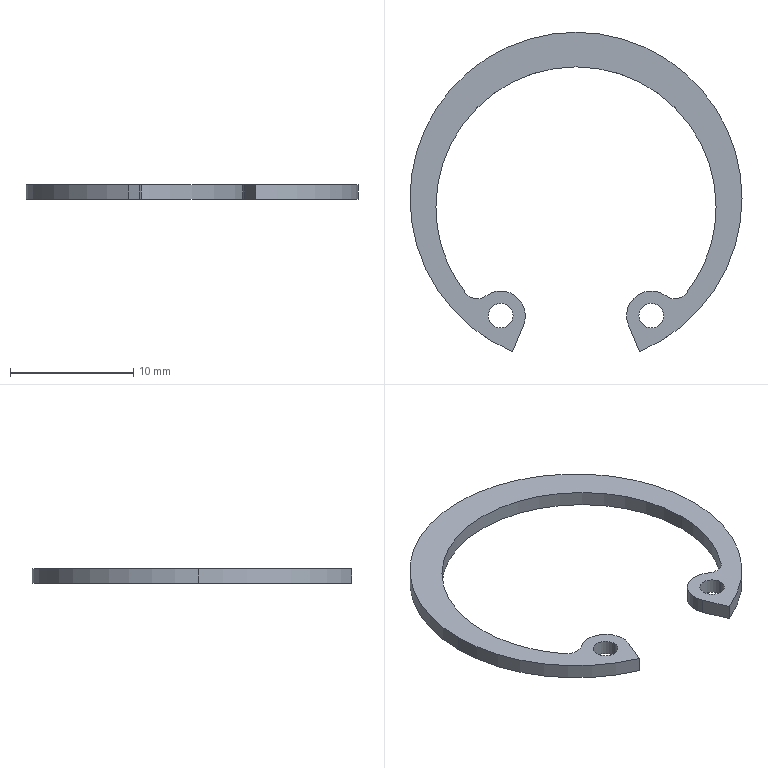Part | STEP file | circlips for holes--type a gb(GB_CONNECTING_PIECE_RING_RRH 25) | 1 solid | 19 faces | box 26.9 x 25.876 x 1.2 mm | volume 193.354 mm3 | cylinder 15 | plane 4 | commonest cylinder face diameters 2 x4 4 x3 22.7 x3 26.9 x3 2.4 x2
STEP:
#1=CARTESIAN_POINT('',(-7.104,-9.51,-1.2));
#2=VERTEX_POINT('',#1);
#3=CARTESIAN_POINT('',(-5.104,-9.51,-1.2));
#4=VERTEX_POINT('',#3);
#5=CARTESIAN_POINT('',(-6.104,-9.51,-1.2));
#6=DIRECTION('',(0.,0.,1.));
#7=DIRECTION('',(1.,0.,0.));
#8=AXIS2_PLACEMENT_3D('',#5,#6,#7);
#9=CIRCLE('',#8,1.);
#10=EDGE_CURVE('',#2,#4,#9,.T.);
#11=ORIENTED_EDGE('',*,*,#10,.F.);
#12=CARTESIAN_POINT('',(-7.104,-9.51,0.));
#13=VERTEX_POINT('',#12);
#14=CARTESIAN_POINT('',(-7.104,-9.51,-1.2));
#15=DIRECTION('',(0.,0.,1.));
#16=VECTOR('',#15,1000.);
#17=LINE('',#14,#16);
#18=EDGE_CURVE('',#2,#13,#17,.T.);
#19=ORIENTED_EDGE('',*,*,#18,.T.);
#20=CARTESIAN_POINT('',(-5.104,-9.51,0.));
#21=VERTEX_POINT('',#20);
#22=CARTESIAN_POINT('',(-6.104,-9.51,0.));
#23=DIRECTION('',(0.,0.,1.));
#24=DIRECTION('',(1.,0.,0.));
#25=AXIS2_PLACEMENT_3D('',#22,#23,#24);
#26=CIRCLE('',#25,1.);
#27=EDGE_CURVE('',#13,#21,#26,.T.);
#28=ORIENTED_EDGE('',*,*,#27,.T.);
#29=CARTESIAN_POINT('',(-5.104,-9.51,-1.2));
#30=DIRECTION('',(0.,0.,1.));
#31=VECTOR('',#30,1000.);
#32=LINE('',#29,#31);
#33=EDGE_CURVE('',#4,#21,#32,.T.);
#34=ORIENTED_EDGE('',*,*,#33,.F.);
#35=EDGE_LOOP('',(#11,#19,#28,#34));
#36=FACE_OUTER_BOUND('',#35,.T.);
#37=CARTESIAN_POINT('',(-6.104,-9.51,-1.2));
#38=DIRECTION('',(0.,0.,1.));
#39=DIRECTION('',(1.,0.,0.));
#40=AXIS2_PLACEMENT_3D('',#37,#38,#39);
#41=CYLINDRICAL_SURFACE('',#40,1.);
#42=ADVANCED_FACE('',(#36),#41,.F.);
#43=CARTESIAN_POINT('',(5.104,-9.51,-1.2));
#44=VERTEX_POINT('',#43);
#45=CARTESIAN_POINT('',(7.104,-9.51,-1.2));
#46=VERTEX_POINT('',#45);
#47=CARTESIAN_POINT('',(6.104,-9.51,-1.2));
#48=DIRECTION('',(0.,0.,1.));
#49=DIRECTION('',(-1.,0.,0.));
#50=AXIS2_PLACEMENT_3D('',#47,#48,#49);
#51=CIRCLE('',#50,1.);
#52=EDGE_CURVE('',#44,#46,#51,.T.);
#53=ORIENTED_EDGE('',*,*,#52,.F.);
#54=CARTESIAN_POINT('',(5.104,-9.51,0.));
#55=VERTEX_POINT('',#54);
#56=CARTESIAN_POINT('',(5.104,-9.51,-1.2));
#57=DIRECTION('',(0.,0.,1.));
#58=VECTOR('',#57,1000.);
#59=LINE('',#56,#58);
#60=EDGE_CURVE('',#44,#55,#59,.T.);
#61=ORIENTED_EDGE('',*,*,#60,.T.);
#62=CARTESIAN_POINT('',(7.104,-9.51,0.));
#63=VERTEX_POINT('',#62);
#64=CARTESIAN_POINT('',(6.104,-9.51,0.));
#65=DIRECTION('',(0.,0.,1.));
#66=DIRECTION('',(-1.,0.,0.));
#67=AXIS2_PLACEMENT_3D('',#64,#65,#66);
#68=CIRCLE('',#67,1.);
#69=EDGE_CURVE('',#55,#63,#68,.T.);
#70=ORIENTED_EDGE('',*,*,#69,.T.);
#71=CARTESIAN_POINT('',(7.104,-9.51,-1.2));
#72=DIRECTION('',(0.,0.,1.));
#73=VECTOR('',#72,1000.);
#74=LINE('',#71,#73);
#75=EDGE_CURVE('',#46,#63,#74,.T.);
#76=ORIENTED_EDGE('',*,*,#75,.F.);
#77=EDGE_LOOP('',(#53,#61,#70,#76));
#78=FACE_OUTER_BOUND('',#77,.T.);
#79=CARTESIAN_POINT('',(6.104,-9.51,-1.2));
#80=DIRECTION('',(0.,0.,1.));
#81=DIRECTION('',(1.,0.,0.));
#82=AXIS2_PLACEMENT_3D('',#79,#80,#81);
#83=CYLINDRICAL_SURFACE('',#82,1.);
#84=ADVANCED_FACE('',(#78),#83,.F.);
#85=CARTESIAN_POINT('',(-4.256,-10.275,-1.2));
#86=VERTEX_POINT('',#85);
#87=CARTESIAN_POINT('',(-4.104,-9.51,-1.2));
#88=VERTEX_POINT('',#87);
#89=CARTESIAN_POINT('',(-6.104,-9.51,-1.2));
#90=DIRECTION('',(0.,0.,1.));
#91=DIRECTION('',(1.,0.,0.));
#92=AXIS2_PLACEMENT_3D('',#89,#90,#91);
#93=CIRCLE('',#92,2.);
#94=EDGE_CURVE('',#86,#88,#93,.T.);
#95=ORIENTED_EDGE('',*,*,#94,.T.);
#96=CARTESIAN_POINT('',(-4.104,-9.51,0.));
#97=VERTEX_POINT('',#96);
#98=CARTESIAN_POINT('',(-4.104,-9.51,-1.2));
#99=DIRECTION('',(0.,0.,1.));
#100=VECTOR('',#99,1000.);
#101=LINE('',#98,#100);
#102=EDGE_CURVE('',#88,#97,#101,.T.);
#103=ORIENTED_EDGE('',*,*,#102,.T.);
#104=CARTESIAN_POINT('',(-4.256,-10.275,0.));
#105=VERTEX_POINT('',#104);
#106=CARTESIAN_POINT('',(-6.104,-9.51,0.));
#107=DIRECTION('',(0.,0.,1.));
#108=DIRECTION('',(1.,0.,0.));
#109=AXIS2_PLACEMENT_3D('',#106,#107,#108);
#110=CIRCLE('',#109,2.);
#111=EDGE_CURVE('',#105,#97,#110,.T.);
#112=ORIENTED_EDGE('',*,*,#111,.F.);
#113=CARTESIAN_POINT('',(-4.256,-10.275,-1.2));
#114=DIRECTION('',(0.,0.,1.));
#115=VECTOR('',#114,1000.);
#116=LINE('',#113,#115);
#117=EDGE_CURVE('',#86,#105,#116,.T.);
#118=ORIENTED_EDGE('',*,*,#117,.F.);
#119=EDGE_LOOP('',(#95,#103,#112,#118));
#120=FACE_OUTER_BOUND('',#119,.T.);
#121=CARTESIAN_POINT('',(-6.104,-9.51,-1.2));
#122=DIRECTION('',(0.,0.,1.));
#123=DIRECTION('',(1.,0.,0.));
#124=AXIS2_PLACEMENT_3D('',#121,#122,#123);
#125=CYLINDRICAL_SURFACE('',#124,2.);
#126=ADVANCED_FACE('',(#120),#125,.T.);
#127=CARTESIAN_POINT('',(-8.954,-7.675,-1.2));
#128=VERTEX_POINT('',#127);
#129=CARTESIAN_POINT('',(-11.35,-0.7,-1.2));
#130=VERTEX_POINT('',#129);
#131=CARTESIAN_POINT('',(0.,-0.7,-1.2));
#132=DIRECTION('',(0.,0.,-1.));
#133=DIRECTION('',(1.,0.,0.));
#134=AXIS2_PLACEMENT_3D('',#131,#132,#133);
#135=CIRCLE('',#134,11.35);
#136=EDGE_CURVE('',#128,#130,#135,.T.);
#137=ORIENTED_EDGE('',*,*,#136,.T.);
#138=CARTESIAN_POINT('',(-11.35,-0.7,0.));
#139=VERTEX_POINT('',#138);
#140=CARTESIAN_POINT('',(-11.35,-0.7,-1.2));
#141=DIRECTION('',(0.,0.,1.));
#142=VECTOR('',#141,1000.);
#143=LINE('',#140,#142);
#144=EDGE_CURVE('',#130,#139,#143,.T.);
#145=ORIENTED_EDGE('',*,*,#144,.T.);
#146=CARTESIAN_POINT('',(-8.954,-7.675,0.));
#147=VERTEX_POINT('',#146);
#148=CARTESIAN_POINT('',(0.,-0.7,0.));
#149=DIRECTION('',(0.,0.,-1.));
#150=DIRECTION('',(1.,0.,0.));
#151=AXIS2_PLACEMENT_3D('',#148,#149,#150);
#152=CIRCLE('',#151,11.35);
#153=EDGE_CURVE('',#147,#139,#152,.T.);
#154=ORIENTED_EDGE('',*,*,#153,.F.);
#155=CARTESIAN_POINT('',(-8.954,-7.675,-1.2));
#156=DIRECTION('',(0.,0.,1.));
#157=VECTOR('',#156,1000.);
#158=LINE('',#155,#157);
#159=EDGE_CURVE('',#128,#147,#158,.T.);
#160=ORIENTED_EDGE('',*,*,#159,.F.);
#161=EDGE_LOOP('',(#137,#145,#154,#160));
#162=FACE_OUTER_BOUND('',#161,.T.);
#163=CARTESIAN_POINT('',(0.,-0.7,-1.2));
#164=DIRECTION('',(0.,0.,1.));
#165=DIRECTION('',(1.,0.,0.));
#166=AXIS2_PLACEMENT_3D('',#163,#164,#165);
#167=CYLINDRICAL_SURFACE('',#166,11.35);
#168=ADVANCED_FACE('',(#162),#167,.F.);
#169=ORIENTED_EDGE('',*,*,#144,.F.);
#170=CARTESIAN_POINT('',(11.35,-0.7,-1.2));
#171=VERTEX_POINT('',#170);
#172=CARTESIAN_POINT('',(0.,-0.7,-1.2));
#173=DIRECTION('',(0.,0.,-1.));
#174=DIRECTION('',(1.,0.,0.));
#175=AXIS2_PLACEMENT_3D('',#172,#173,#174);
#176=CIRCLE('',#175,11.35);
#177=EDGE_CURVE('',#130,#171,#176,.T.);
#178=ORIENTED_EDGE('',*,*,#177,.T.);
#179=CARTESIAN_POINT('',(11.35,-0.7,0.));
#180=VERTEX_POINT('',#179);
#181=CARTESIAN_POINT('',(11.35,-0.7,-1.2));
#182=DIRECTION('',(0.,0.,1.));
#183=VECTOR('',#182,1000.);
#184=LINE('',#181,#183);
#185=EDGE_CURVE('',#171,#180,#184,.T.);
#186=ORIENTED_EDGE('',*,*,#185,.T.);
#187=CARTESIAN_POINT('',(0.,-0.7,0.));
#188=DIRECTION('',(0.,0.,-1.));
#189=DIRECTION('',(1.,0.,0.));
#190=AXIS2_PLACEMENT_3D('',#187,#188,#189);
#191=CIRCLE('',#190,11.35);
#192=EDGE_CURVE('',#139,#180,#191,.T.);
#193=ORIENTED_EDGE('',*,*,#192,.F.);
#194=EDGE_LOOP('',(#169,#178,#186,#193));
#195=FACE_OUTER_BOUND('',#194,.T.);
#196=CARTESIAN_POINT('',(0.,-0.7,-1.2));
#197=DIRECTION('',(0.,0.,1.));
#198=DIRECTION('',(1.,0.,0.));
#199=AXIS2_PLACEMENT_3D('',#196,#197,#198);
#200=CYLINDRICAL_SURFACE('',#199,11.35);
#201=ADVANCED_FACE('',(#195),#200,.F.);
#202=CARTESIAN_POINT('',(13.45,0.,-1.2));
#203=VERTEX_POINT('',#202);
#204=CARTESIAN_POINT('',(-13.45,0.,-1.2));
#205=VERTEX_POINT('',#204);
#206=CARTESIAN_POINT('',(0.,0.,-1.2));
#207=DIRECTION('',(0.,0.,1.));
#208=DIRECTION('',(1.,0.,0.));
#209=AXIS2_PLACEMENT_3D('',#206,#207,#208);
#210=CIRCLE('',#209,13.45);
#211=EDGE_CURVE('',#203,#205,#210,.T.);
#212=ORIENTED_EDGE('',*,*,#211,.T.);
#213=CARTESIAN_POINT('',(-13.45,0.,0.));
#214=VERTEX_POINT('',#213);
#215=CARTESIAN_POINT('',(-13.45,0.,-1.2));
#216=DIRECTION('',(0.,0.,1.));
#217=VECTOR('',#216,1000.);
#218=LINE('',#215,#217);
#219=EDGE_CURVE('',#205,#214,#218,.T.);
#220=ORIENTED_EDGE('',*,*,#219,.T.);
#221=CARTESIAN_POINT('',(13.45,0.,0.));
#222=VERTEX_POINT('',#221);
#223=CARTESIAN_POINT('',(0.,0.,0.));
#224=DIRECTION('',(0.,0.,1.));
#225=DIRECTION('',(1.,0.,0.));
#226=AXIS2_PLACEMENT_3D('',#223,#224,#225);
#227=CIRCLE('',#226,13.45);
#228=EDGE_CURVE('',#222,#214,#227,.T.);
#229=ORIENTED_EDGE('',*,*,#228,.F.);
#230=CARTESIAN_POINT('',(13.45,0.,-1.2));
#231=DIRECTION('',(0.,0.,1.));
#232=VECTOR('',#231,1000.);
#233=LINE('',#230,#232);
#234=EDGE_CURVE('',#203,#222,#233,.T.);
#235=ORIENTED_EDGE('',*,*,#234,.F.);
#236=EDGE_LOOP('',(#212,#220,#229,#235));
#237=FACE_OUTER_BOUND('',#236,.T.);
#238=CARTESIAN_POINT('',(0.,0.,-1.2));
#239=DIRECTION('',(0.,0.,1.));
#240=DIRECTION('',(1.,0.,0.));
#241=AXIS2_PLACEMENT_3D('',#238,#239,#240);
#242=CYLINDRICAL_SURFACE('',#241,13.45);
#243=ADVANCED_FACE('',(#237),#242,.T.);
#244=CARTESIAN_POINT('',(5.147,-12.426,-1.2));
#245=VERTEX_POINT('',#244);
#246=CARTESIAN_POINT('',(0.,0.,-1.2));
#247=DIRECTION('',(0.,0.,1.));
#248=DIRECTION('',(1.,0.,0.));
#249=AXIS2_PLACEMENT_3D('',#246,#247,#248);
#250=CIRCLE('',#249,13.45);
#251=EDGE_CURVE('',#245,#203,#250,.T.);
#252=ORIENTED_EDGE('',*,*,#251,.T.);
#253=ORIENTED_EDGE('',*,*,#234,.T.);
#254=CARTESIAN_POINT('',(5.147,-12.426,0.));
#255=VERTEX_POINT('',#254);
#256=CARTESIAN_POINT('',(0.,0.,0.));
#257=DIRECTION('',(0.,0.,1.));
#258=DIRECTION('',(1.,0.,0.));
#259=AXIS2_PLACEMENT_3D('',#256,#257,#258);
#260=CIRCLE('',#259,13.45);
#261=EDGE_CURVE('',#255,#222,#260,.T.);
#262=ORIENTED_EDGE('',*,*,#261,.F.);
#263=CARTESIAN_POINT('',(5.147,-12.426,-1.2));
#264=DIRECTION('',(0.,0.,1.));
#265=VECTOR('',#264,1000.);
#266=LINE('',#263,#265);
#267=EDGE_CURVE('',#245,#255,#266,.T.);
#268=ORIENTED_EDGE('',*,*,#267,.F.);
#269=EDGE_LOOP('',(#252,#253,#262,#268));
#270=FACE_OUTER_BOUND('',#269,.T.);
#271=CARTESIAN_POINT('',(0.,0.,-1.2));
#272=DIRECTION('',(0.,0.,1.));
#273=DIRECTION('',(1.,0.,0.));
#274=AXIS2_PLACEMENT_3D('',#271,#272,#273);
#275=CYLINDRICAL_SURFACE('',#274,13.45);
#276=ADVANCED_FACE('',(#270),#275,.T.);
#277=ORIENTED_EDGE('',*,*,#219,.F.);
#278=CARTESIAN_POINT('',(-5.147,-12.426,-1.2));
#279=VERTEX_POINT('',#278);
#280=CARTESIAN_POINT('',(0.,0.,-1.2));
#281=DIRECTION('',(0.,0.,1.));
#282=DIRECTION('',(1.,0.,0.));
#283=AXIS2_PLACEMENT_3D('',#280,#281,#282);
#284=CIRCLE('',#283,13.45);
#285=EDGE_CURVE('',#205,#279,#284,.T.);
#286=ORIENTED_EDGE('',*,*,#285,.T.);
#287=CARTESIAN_POINT('',(-5.147,-12.426,0.));
#288=VERTEX_POINT('',#287);
#289=CARTESIAN_POINT('',(-5.147,-12.426,-1.2));
#290=DIRECTION('',(0.,0.,1.));
#291=VECTOR('',#290,1000.);
#292=LINE('',#289,#291);
#293=EDGE_CURVE('',#279,#288,#292,.T.);
#294=ORIENTED_EDGE('',*,*,#293,.T.);
#295=CARTESIAN_POINT('',(0.,0.,0.));
#296=DIRECTION('',(0.,0.,1.));
#297=DIRECTION('',(1.,0.,0.));
#298=AXIS2_PLACEMENT_3D('',#295,#296,#297);
#299=CIRCLE('',#298,13.45);
#300=EDGE_CURVE('',#214,#288,#299,.T.);
#301=ORIENTED_EDGE('',*,*,#300,.F.);
#302=EDGE_LOOP('',(#277,#286,#294,#301));
#303=FACE_OUTER_BOUND('',#302,.T.);
#304=CARTESIAN_POINT('',(0.,0.,-1.2));
#305=DIRECTION('',(0.,0.,1.));
#306=DIRECTION('',(1.,0.,0.));
#307=AXIS2_PLACEMENT_3D('',#304,#305,#306);
#308=CYLINDRICAL_SURFACE('',#307,13.45);
#309=ADVANCED_FACE('',(#303),#308,.T.);
#310=CARTESIAN_POINT('',(4.256,-10.275,0.));
#311=VERTEX_POINT('',#310);
#312=CARTESIAN_POINT('',(4.256,-10.275,0.));
#313=DIRECTION('',(0.3827,-0.9239,0.));
#314=VECTOR('',#313,1000.);
#315=LINE('',#312,#314);
#316=EDGE_CURVE('',#311,#255,#315,.T.);
#317=ORIENTED_EDGE('',*,*,#316,.F.);
#318=CARTESIAN_POINT('',(4.256,-10.275,-1.2));
#319=VERTEX_POINT('',#318);
#320=CARTESIAN_POINT('',(4.256,-10.275,-1.2));
#321=DIRECTION('',(0.,0.,1.));
#322=VECTOR('',#321,1000.);
#323=LINE('',#320,#322);
#324=EDGE_CURVE('',#319,#311,#323,.T.);
#325=ORIENTED_EDGE('',*,*,#324,.F.);
#326=CARTESIAN_POINT('',(4.256,-10.275,-1.2));
#327=DIRECTION('',(0.3827,-0.9239,0.));
#328=VECTOR('',#327,1000.);
#329=LINE('',#326,#328);
#330=EDGE_CURVE('',#319,#245,#329,.T.);
#331=ORIENTED_EDGE('',*,*,#330,.T.);
#332=ORIENTED_EDGE('',*,*,#267,.T.);
#333=EDGE_LOOP('',(#317,#325,#331,#332));
#334=FACE_OUTER_BOUND('',#333,.T.);
#335=CARTESIAN_POINT('',(4.256,-10.275,-1.2));
#336=DIRECTION('',(-0.9239,-0.3827,0.));
#337=DIRECTION('',(0.3827,-0.9239,0.));
#338=AXIS2_PLACEMENT_3D('',#335,#336,#337);
#339=PLANE('',#338);
#340=ADVANCED_FACE('',(#334),#339,.T.);
#341=CARTESIAN_POINT('',(7.294,-7.902,0.));
#342=VERTEX_POINT('',#341);
#343=CARTESIAN_POINT('',(6.104,-9.51,0.));
#344=DIRECTION('',(0.,0.,1.));
#345=DIRECTION('',(-1.,0.,0.));
#346=AXIS2_PLACEMENT_3D('',#343,#344,#345);
#347=CIRCLE('',#346,2.);
#348=EDGE_CURVE('',#342,#311,#347,.T.);
#349=ORIENTED_EDGE('',*,*,#348,.F.);
#350=CARTESIAN_POINT('',(7.294,-7.902,-1.2));
#351=VERTEX_POINT('',#350);
#352=CARTESIAN_POINT('',(7.294,-7.902,-1.2));
#353=DIRECTION('',(0.,0.,1.));
#354=VECTOR('',#353,1000.);
#355=LINE('',#352,#354);
#356=EDGE_CURVE('',#351,#342,#355,.T.);
#357=ORIENTED_EDGE('',*,*,#356,.F.);
#358=CARTESIAN_POINT('',(6.104,-9.51,-1.2));
#359=DIRECTION('',(0.,0.,1.));
#360=DIRECTION('',(-1.,0.,0.));
#361=AXIS2_PLACEMENT_3D('',#358,#359,#360);
#362=CIRCLE('',#361,2.);
#363=EDGE_CURVE('',#351,#319,#362,.T.);
#364=ORIENTED_EDGE('',*,*,#363,.T.);
#365=ORIENTED_EDGE('',*,*,#324,.T.);
#366=EDGE_LOOP('',(#349,#357,#364,#365));
#367=FACE_OUTER_BOUND('',#366,.T.);
#368=CARTESIAN_POINT('',(6.104,-9.51,-1.2));
#369=DIRECTION('',(0.,0.,1.));
#370=DIRECTION('',(1.,0.,0.));
#371=AXIS2_PLACEMENT_3D('',#368,#369,#370);
#372=CYLINDRICAL_SURFACE('',#371,2.);
#373=ADVANCED_FACE('',(#367),#372,.T.);
#374=CARTESIAN_POINT('',(8.954,-7.675,0.));
#375=VERTEX_POINT('',#374);
#376=CARTESIAN_POINT('',(8.007,-6.937,0.));
#377=DIRECTION('',(0.,0.,-1.));
#378=DIRECTION('',(-1.,0.,0.));
#379=AXIS2_PLACEMENT_3D('',#376,#377,#378);
#380=CIRCLE('',#379,1.2);
#381=EDGE_CURVE('',#375,#342,#380,.T.);
#382=ORIENTED_EDGE('',*,*,#381,.F.);
#383=CARTESIAN_POINT('',(8.954,-7.675,-1.2));
#384=VERTEX_POINT('',#383);
#385=CARTESIAN_POINT('',(8.954,-7.675,-1.2));
#386=DIRECTION('',(0.,0.,1.));
#387=VECTOR('',#386,1000.);
#388=LINE('',#385,#387);
#389=EDGE_CURVE('',#384,#375,#388,.T.);
#390=ORIENTED_EDGE('',*,*,#389,.F.);
#391=CARTESIAN_POINT('',(8.007,-6.937,-1.2));
#392=DIRECTION('',(0.,0.,-1.));
#393=DIRECTION('',(-1.,0.,0.));
#394=AXIS2_PLACEMENT_3D('',#391,#392,#393);
#395=CIRCLE('',#394,1.2);
#396=EDGE_CURVE('',#384,#351,#395,.T.);
#397=ORIENTED_EDGE('',*,*,#396,.T.);
#398=ORIENTED_EDGE('',*,*,#356,.T.);
#399=EDGE_LOOP('',(#382,#390,#397,#398));
#400=FACE_OUTER_BOUND('',#399,.T.);
#401=CARTESIAN_POINT('',(8.007,-6.937,-1.2));
#402=DIRECTION('',(0.,0.,1.));
#403=DIRECTION('',(1.,0.,0.));
#404=AXIS2_PLACEMENT_3D('',#401,#402,#403);
#405=CYLINDRICAL_SURFACE('',#404,1.2);
#406=ADVANCED_FACE('',(#400),#405,.F.);
#407=ORIENTED_EDGE('',*,*,#185,.F.);
#408=CARTESIAN_POINT('',(0.,-0.7,-1.2));
#409=DIRECTION('',(0.,0.,-1.));
#410=DIRECTION('',(1.,0.,0.));
#411=AXIS2_PLACEMENT_3D('',#408,#409,#410);
#412=CIRCLE('',#411,11.35);
#413=EDGE_CURVE('',#171,#384,#412,.T.);
#414=ORIENTED_EDGE('',*,*,#413,.T.);
#415=ORIENTED_EDGE('',*,*,#389,.T.);
#416=CARTESIAN_POINT('',(0.,-0.7,0.));
#417=DIRECTION('',(0.,0.,-1.));
#418=DIRECTION('',(1.,0.,0.));
#419=AXIS2_PLACEMENT_3D('',#416,#417,#418);
#420=CIRCLE('',#419,11.35);
#421=EDGE_CURVE('',#180,#375,#420,.T.);
#422=ORIENTED_EDGE('',*,*,#421,.F.);
#423=EDGE_LOOP('',(#407,#414,#415,#422));
#424=FACE_OUTER_BOUND('',#423,.T.);
#425=CARTESIAN_POINT('',(0.,-0.7,-1.2));
#426=DIRECTION('',(0.,0.,1.));
#427=DIRECTION('',(1.,0.,0.));
#428=AXIS2_PLACEMENT_3D('',#425,#426,#427);
#429=CYLINDRICAL_SURFACE('',#428,11.35);
#430=ADVANCED_FACE('',(#424),#429,.F.);
#431=CARTESIAN_POINT('',(-7.294,-7.902,0.));
#432=VERTEX_POINT('',#431);
#433=CARTESIAN_POINT('',(-8.007,-6.937,0.));
#434=DIRECTION('',(0.,0.,-1.));
#435=DIRECTION('',(1.,0.,0.));
#436=AXIS2_PLACEMENT_3D('',#433,#434,#435);
#437=CIRCLE('',#436,1.2);
#438=EDGE_CURVE('',#432,#147,#437,.T.);
#439=ORIENTED_EDGE('',*,*,#438,.F.);
#440=CARTESIAN_POINT('',(-7.294,-7.902,-1.2));
#441=VERTEX_POINT('',#440);
#442=CARTESIAN_POINT('',(-7.294,-7.902,-1.2));
#443=DIRECTION('',(0.,0.,1.));
#444=VECTOR('',#443,1000.);
#445=LINE('',#442,#444);
#446=EDGE_CURVE('',#441,#432,#445,.T.);
#447=ORIENTED_EDGE('',*,*,#446,.F.);
#448=CARTESIAN_POINT('',(-8.007,-6.937,-1.2));
#449=DIRECTION('',(0.,0.,-1.));
#450=DIRECTION('',(1.,0.,0.));
#451=AXIS2_PLACEMENT_3D('',#448,#449,#450);
#452=CIRCLE('',#451,1.2);
#453=EDGE_CURVE('',#441,#128,#452,.T.);
#454=ORIENTED_EDGE('',*,*,#453,.T.);
#455=ORIENTED_EDGE('',*,*,#159,.T.);
#456=EDGE_LOOP('',(#439,#447,#454,#455));
#457=FACE_OUTER_BOUND('',#456,.T.);
#458=CARTESIAN_POINT('',(-8.007,-6.937,-1.2));
#459=DIRECTION('',(0.,0.,1.));
#460=DIRECTION('',(1.,0.,0.));
#461=AXIS2_PLACEMENT_3D('',#458,#459,#460);
#462=CYLINDRICAL_SURFACE('',#461,1.2);
#463=ADVANCED_FACE('',(#457),#462,.F.);
#464=ORIENTED_EDGE('',*,*,#102,.F.);
#465=CARTESIAN_POINT('',(-6.104,-9.51,-1.2));
#466=DIRECTION('',(0.,0.,1.));
#467=DIRECTION('',(1.,0.,0.));
#468=AXIS2_PLACEMENT_3D('',#465,#466,#467);
#469=CIRCLE('',#468,2.);
#470=EDGE_CURVE('',#88,#441,#469,.T.);
#471=ORIENTED_EDGE('',*,*,#470,.T.);
#472=ORIENTED_EDGE('',*,*,#446,.T.);
#473=CARTESIAN_POINT('',(-6.104,-9.51,0.));
#474=DIRECTION('',(0.,0.,1.));
#475=DIRECTION('',(1.,0.,0.));
#476=AXIS2_PLACEMENT_3D('',#473,#474,#475);
#477=CIRCLE('',#476,2.);
#478=EDGE_CURVE('',#97,#432,#477,.T.);
#479=ORIENTED_EDGE('',*,*,#478,.F.);
#480=EDGE_LOOP('',(#464,#471,#472,#479));
#481=FACE_OUTER_BOUND('',#480,.T.);
#482=CARTESIAN_POINT('',(-6.104,-9.51,-1.2));
#483=DIRECTION('',(0.,0.,1.));
#484=DIRECTION('',(1.,0.,0.));
#485=AXIS2_PLACEMENT_3D('',#482,#483,#484);
#486=CYLINDRICAL_SURFACE('',#485,2.);
#487=ADVANCED_FACE('',(#481),#486,.T.);
#488=CARTESIAN_POINT('',(-4.256,-10.275,0.));
#489=DIRECTION('',(0.3827,0.9239,0.));
#490=VECTOR('',#489,1000.);
#491=LINE('',#488,#490);
#492=EDGE_CURVE('',#288,#105,#491,.T.);
#493=ORIENTED_EDGE('',*,*,#492,.F.);
#494=ORIENTED_EDGE('',*,*,#293,.F.);
#495=CARTESIAN_POINT('',(-4.256,-10.275,-1.2));
#496=DIRECTION('',(0.3827,0.9239,0.));
#497=VECTOR('',#496,1000.);
#498=LINE('',#495,#497);
#499=EDGE_CURVE('',#279,#86,#498,.T.);
#500=ORIENTED_EDGE('',*,*,#499,.T.);
#501=ORIENTED_EDGE('',*,*,#117,.T.);
#502=EDGE_LOOP('',(#493,#494,#500,#501));
#503=FACE_OUTER_BOUND('',#502,.T.);
#504=CARTESIAN_POINT('',(-4.256,-10.275,-1.2));
#505=DIRECTION('',(0.9239,-0.3827,0.));
#506=DIRECTION('',(0.3827,0.9239,0.));
#507=AXIS2_PLACEMENT_3D('',#504,#505,#506);
#508=PLANE('',#507);
#509=ADVANCED_FACE('',(#503),#508,.T.);
#510=CARTESIAN_POINT('',(-6.104,-9.51,-1.2));
#511=DIRECTION('',(0.,0.,1.));
#512=DIRECTION('',(1.,0.,0.));
#513=AXIS2_PLACEMENT_3D('',#510,#511,#512);
#514=CIRCLE('',#513,1.);
#515=EDGE_CURVE('',#4,#2,#514,.T.);
#516=ORIENTED_EDGE('',*,*,#515,.T.);
#517=ORIENTED_EDGE('',*,*,#10,.T.);
#518=EDGE_LOOP('',(#516,#517));
#519=FACE_BOUND('',#518,.T.);
#520=CARTESIAN_POINT('',(6.104,-9.51,-1.2));
#521=DIRECTION('',(0.,0.,1.));
#522=DIRECTION('',(-1.,0.,0.));
#523=AXIS2_PLACEMENT_3D('',#520,#521,#522);
#524=CIRCLE('',#523,1.);
#525=EDGE_CURVE('',#46,#44,#524,.T.);
#526=ORIENTED_EDGE('',*,*,#525,.T.);
#527=ORIENTED_EDGE('',*,*,#52,.T.);
#528=EDGE_LOOP('',(#526,#527));
#529=FACE_BOUND('',#528,.T.);
#530=ORIENTED_EDGE('',*,*,#251,.F.);
#531=ORIENTED_EDGE('',*,*,#330,.F.);
#532=ORIENTED_EDGE('',*,*,#363,.F.);
#533=ORIENTED_EDGE('',*,*,#396,.F.);
#534=ORIENTED_EDGE('',*,*,#413,.F.);
#535=ORIENTED_EDGE('',*,*,#177,.F.);
#536=ORIENTED_EDGE('',*,*,#136,.F.);
#537=ORIENTED_EDGE('',*,*,#453,.F.);
#538=ORIENTED_EDGE('',*,*,#470,.F.);
#539=ORIENTED_EDGE('',*,*,#94,.F.);
#540=ORIENTED_EDGE('',*,*,#499,.F.);
#541=ORIENTED_EDGE('',*,*,#285,.F.);
#542=ORIENTED_EDGE('',*,*,#211,.F.);
#543=EDGE_LOOP('',(#530,#531,#532,#533,#534,#535,#536,#537,#538,#539,#540,#541,#542));
#544=FACE_OUTER_BOUND('',#543,.T.);
#545=CARTESIAN_POINT('',(0.,0.,-1.2));
#546=DIRECTION('',(0.,0.,1.));
#547=DIRECTION('',(1.,0.,0.));
#548=AXIS2_PLACEMENT_3D('',#545,#546,#547);
#549=PLANE('',#548);
#550=ADVANCED_FACE('',(#519,#529,#544),#549,.F.);
#551=CARTESIAN_POINT('',(-6.104,-9.51,0.));
#552=DIRECTION('',(0.,0.,1.));
#553=DIRECTION('',(1.,0.,0.));
#554=AXIS2_PLACEMENT_3D('',#551,#552,#553);
#555=CIRCLE('',#554,1.);
#556=EDGE_CURVE('',#21,#13,#555,.T.);
#557=ORIENTED_EDGE('',*,*,#556,.F.);
#558=ORIENTED_EDGE('',*,*,#27,.F.);
#559=EDGE_LOOP('',(#557,#558));
#560=FACE_BOUND('',#559,.T.);
#561=CARTESIAN_POINT('',(6.104,-9.51,0.));
#562=DIRECTION('',(0.,0.,1.));
#563=DIRECTION('',(-1.,0.,0.));
#564=AXIS2_PLACEMENT_3D('',#561,#562,#563);
#565=CIRCLE('',#564,1.);
#566=EDGE_CURVE('',#63,#55,#565,.T.);
#567=ORIENTED_EDGE('',*,*,#566,.F.);
#568=ORIENTED_EDGE('',*,*,#69,.F.);
#569=EDGE_LOOP('',(#567,#568));
#570=FACE_BOUND('',#569,.T.);
#571=ORIENTED_EDGE('',*,*,#261,.T.);
#572=ORIENTED_EDGE('',*,*,#228,.T.);
#573=ORIENTED_EDGE('',*,*,#300,.T.);
#574=ORIENTED_EDGE('',*,*,#492,.T.);
#575=ORIENTED_EDGE('',*,*,#111,.T.);
#576=ORIENTED_EDGE('',*,*,#478,.T.);
#577=ORIENTED_EDGE('',*,*,#438,.T.);
#578=ORIENTED_EDGE('',*,*,#153,.T.);
#579=ORIENTED_EDGE('',*,*,#192,.T.);
#580=ORIENTED_EDGE('',*,*,#421,.T.);
#581=ORIENTED_EDGE('',*,*,#381,.T.);
#582=ORIENTED_EDGE('',*,*,#348,.T.);
#583=ORIENTED_EDGE('',*,*,#316,.T.);
#584=EDGE_LOOP('',(#571,#572,#573,#574,#575,#576,#577,#578,#579,#580,#581,#582,#583));
#585=FACE_OUTER_BOUND('',#584,.T.);
#586=CARTESIAN_POINT('',(0.,0.,0.));
#587=DIRECTION('',(0.,0.,1.));
#588=DIRECTION('',(1.,0.,0.));
#589=AXIS2_PLACEMENT_3D('',#586,#587,#588);
#590=PLANE('',#589);
#591=ADVANCED_FACE('',(#560,#570,#585),#590,.T.);
#592=ORIENTED_EDGE('',*,*,#60,.F.);
#593=ORIENTED_EDGE('',*,*,#525,.F.);
#594=ORIENTED_EDGE('',*,*,#75,.T.);
#595=ORIENTED_EDGE('',*,*,#566,.T.);
#596=EDGE_LOOP('',(#592,#593,#594,#595));
#597=FACE_OUTER_BOUND('',#596,.T.);
#598=CARTESIAN_POINT('',(6.104,-9.51,-1.2));
#599=DIRECTION('',(0.,0.,1.));
#600=DIRECTION('',(1.,0.,0.));
#601=AXIS2_PLACEMENT_3D('',#598,#599,#600);
#602=CYLINDRICAL_SURFACE('',#601,1.);
#603=ADVANCED_FACE('',(#597),#602,.F.);
#604=ORIENTED_EDGE('',*,*,#18,.F.);
#605=ORIENTED_EDGE('',*,*,#515,.F.);
#606=ORIENTED_EDGE('',*,*,#33,.T.);
#607=ORIENTED_EDGE('',*,*,#556,.T.);
#608=EDGE_LOOP('',(#604,#605,#606,#607));
#609=FACE_OUTER_BOUND('',#608,.T.);
#610=CARTESIAN_POINT('',(-6.104,-9.51,-1.2));
#611=DIRECTION('',(0.,0.,1.));
#612=DIRECTION('',(1.,0.,0.));
#613=AXIS2_PLACEMENT_3D('',#610,#611,#612);
#614=CYLINDRICAL_SURFACE('',#613,1.);
#615=ADVANCED_FACE('',(#609),#614,.F.);
#616=CLOSED_SHELL('',(#42,#84,#126,#168,#201,#243,#276,#309,#340,#373,#406,#430,#463,#487,#509,#550,#591,#603,#615));
#617=MANIFOLD_SOLID_BREP('',#616);
#618=CARTESIAN_POINT('',(0.,0.,0.));
#619=DIRECTION('',(0.,0.,1.));
#620=DIRECTION('',(1.,0.,0.));
#621=AXIS2_PLACEMENT_3D('',#618,#619,#620);
#622=(LENGTH_UNIT()NAMED_UNIT(*)SI_UNIT(.MILLI.,.METRE.));
#623=UNCERTAINTY_MEASURE_WITH_UNIT(LENGTH_MEASURE(0.00001),#622,'','');
#624=(NAMED_UNIT(*)PLANE_ANGLE_UNIT()SI_UNIT($,.RADIAN.));
#625=(NAMED_UNIT(*)SI_UNIT($,.STERADIAN.)SOLID_ANGLE_UNIT());
#626=(GEOMETRIC_REPRESENTATION_CONTEXT(3)GLOBAL_UNCERTAINTY_ASSIGNED_CONTEXT((#623))GLOBAL_UNIT_ASSIGNED_CONTEXT((#622,#624,#625))REPRESENTATION_CONTEXT('',''));
#627=ADVANCED_BREP_SHAPE_REPRESENTATION('',(#617,#621),#626);